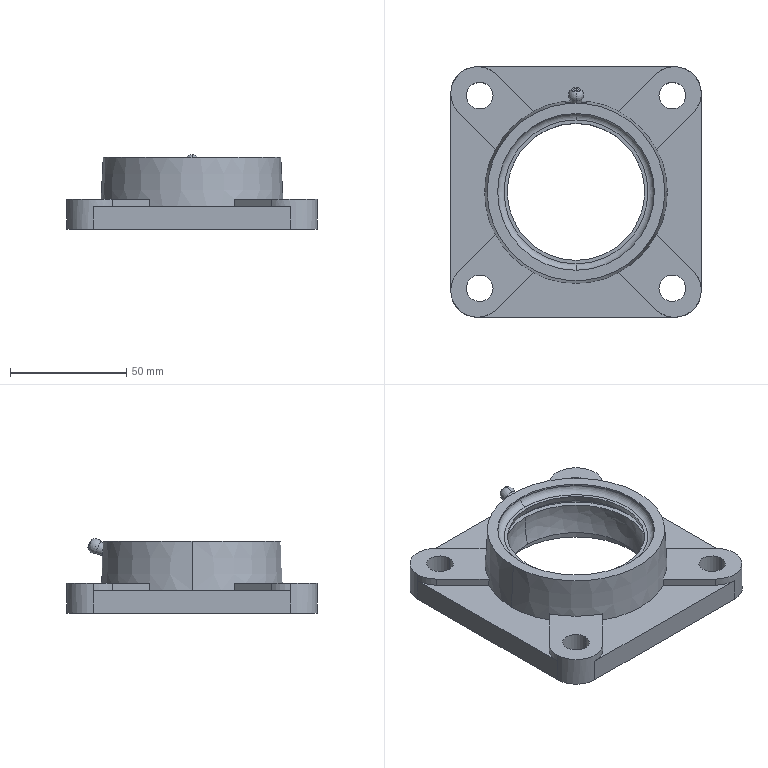Part | SolidWorks | features Boss 2, Cut 1, Extrusion 1, RevCut 1, Revolution 1 | 1 solid | 94 faces | box 108 x 108 x 32.161 mm | volume 104974 mm3 | cylinder 42 | plane 36 | sphere 8 | torus 6 | cone 2 | commonest cylinder face diameters 6 x14 23 x12 11.5 x8 67.58 x4 4.8 x2 65.946 x2